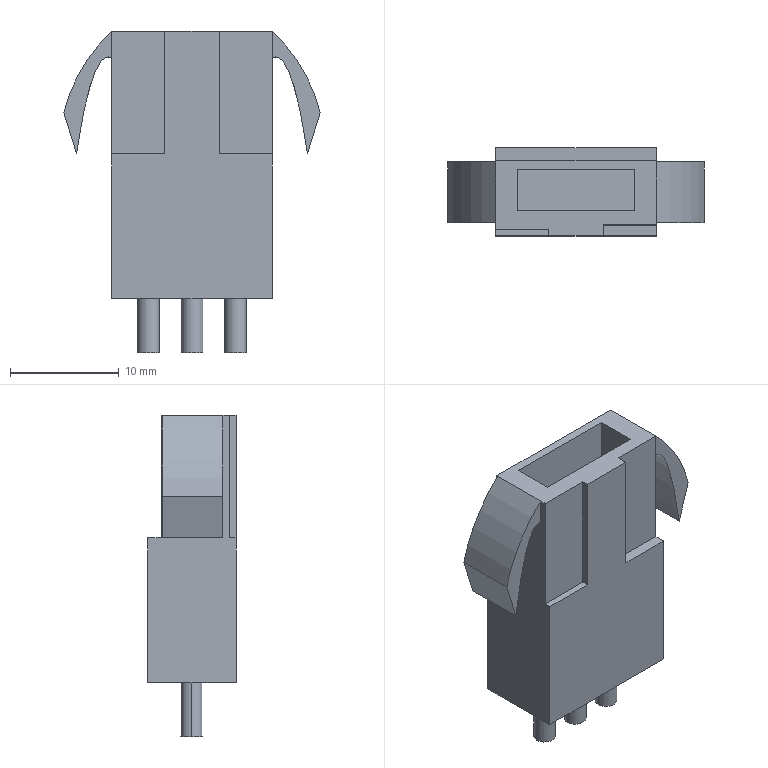Part | STEP file | ELR_03V | 1 solid | 38 faces | box 23.6 x 8.1 x 29.6 mm | volume 2454 mm3 | plane 28 | cylinder 8 | other 2 | commonest cylinder face diameters 2 x6 31.085 x2